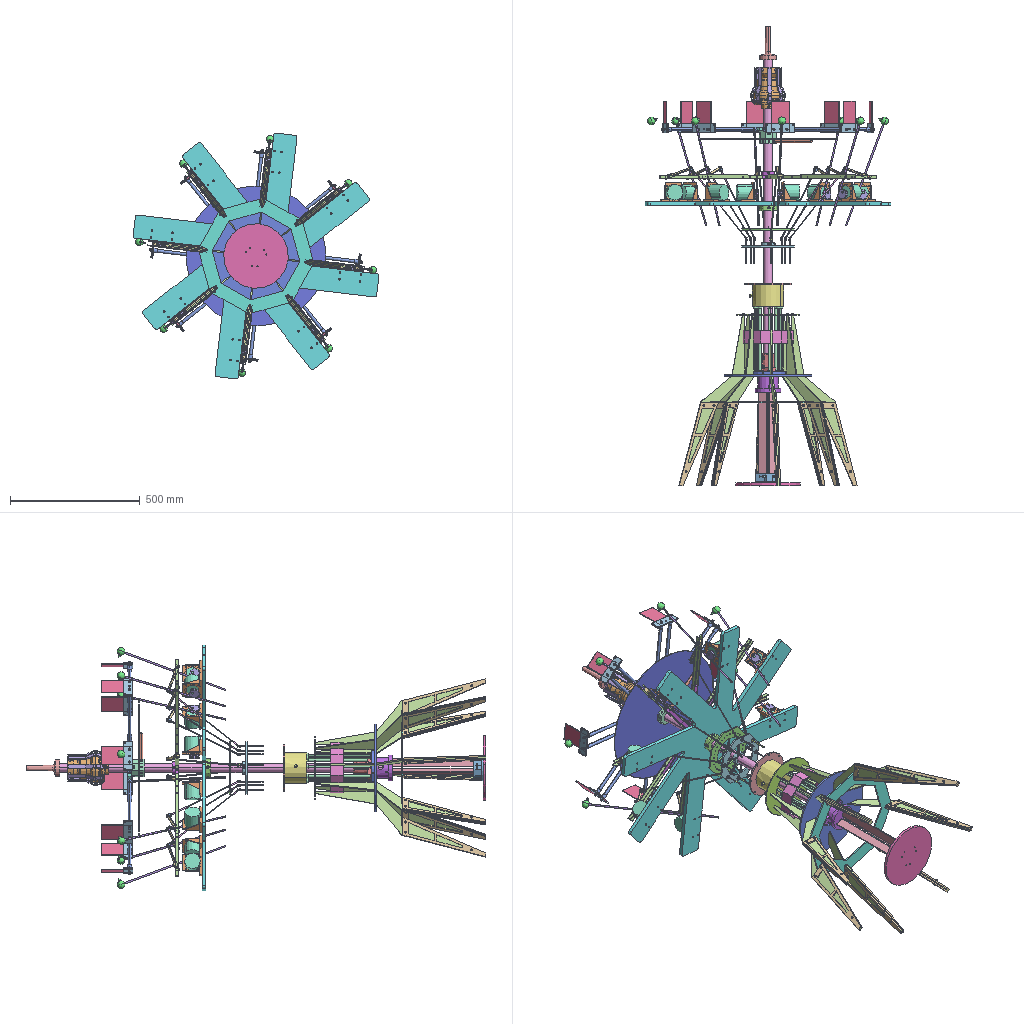Assembly | SolidWorks | 59 different items | 220 placed | box 948 x 1774 x 948 mm
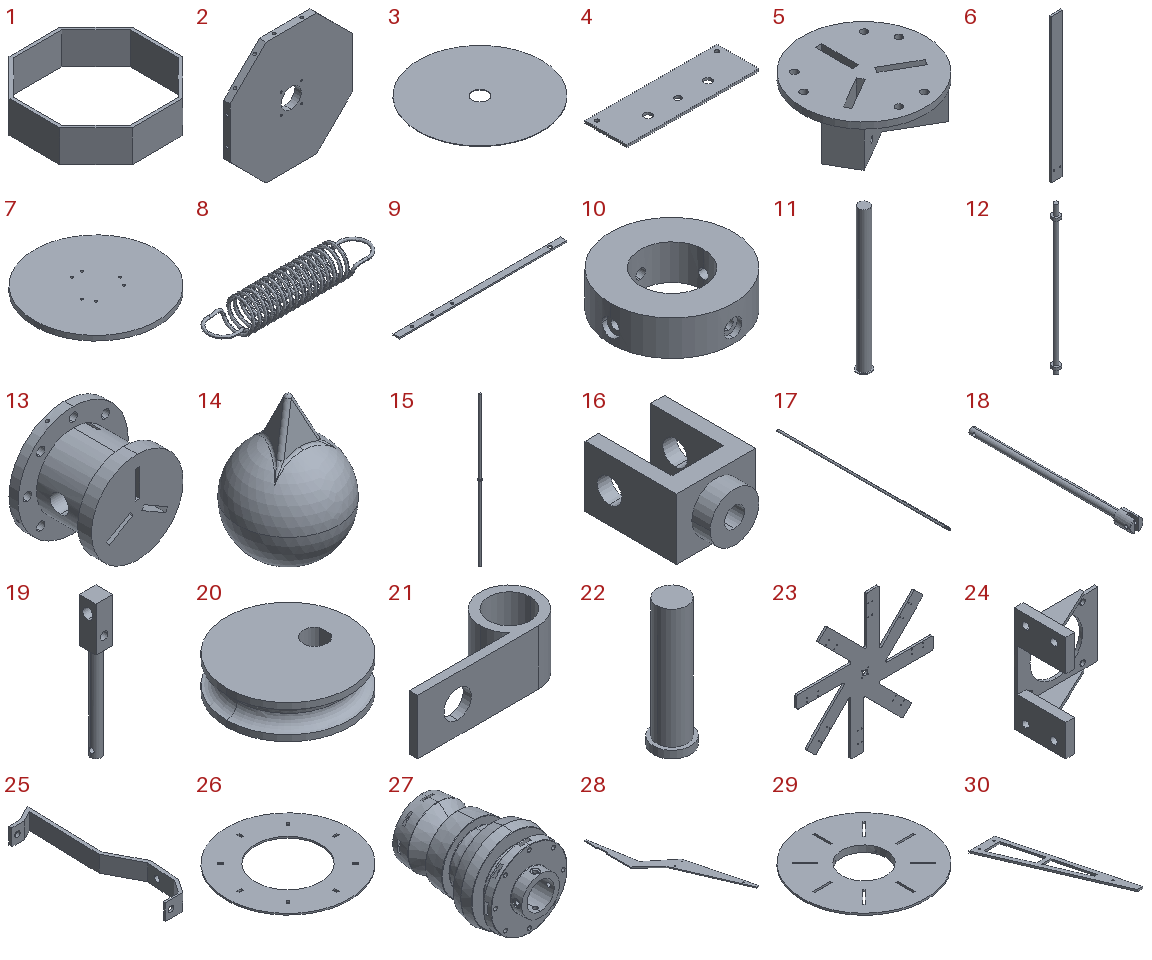Parts list (item | name | quantity | size | volume | features):
1 | - | x1 | 192.167 x 192.167 x 50 mm | 155054 mm3 | features Extrusion 1, ICE 1
2 | - | x1 | 220 x 12 x 220 mm | 463430 mm3 | features ICE 3, CirPattern 2, 3DProfileFeature 1, HoleWzd 1, Revolution 1
3 | - | x1 | 540 x 540 x 2 mm | 450713 mm3 | features Extrusion 1
4 | - | x16 | 110 x 35 x 2 mm | 7490 mm3 | features ICE 3, Extrusion 1
5 | - | x1 | 100 x 100 x 35 mm | 118431 mm3 | features ICE 6, CirPattern 2, Extrusion 1
6 | - | x3 | 30 x 5 x 375 mm | 56098 mm3 | features ICE 4, Cut 1, Extrusion 1, MirrorSolid 1
7 | - | x1 | 250 x 250 x 10 mm | 490035 mm3 | features 3DProfileFeature 1, CirPattern 1, Extrusion 1, HoleWzd 1
8 | - | x1 | 56.999 x 11.387 x 10.999 mm | 441.954 mm3 | features 3DProfileFeature 2, CirPattern 1, CombineBodies 1, Helix 1, ICE 1, Sweep 1
9 | - | x16 | 375 x 14 x 3 mm | 15385 mm3 | features Extrusion 1, ICE 1
10 | - | x1 | 70 x 70 x 20 mm | 54005 mm3 | features CirPattern 2, ICE 2, 3DProfileFeature 1, Extrusion 1, HoleWzd 1
11 | - | x1 | 12.5 x 12.5 x 131 mm | 10333 mm3 | features Extrusion 1, ICE 1
12 | - | x8 | 15 x 15 x 280 mm | 15339 mm3 | features ICE 2, Extrusion 1
13 | - | x1 | 120 x 80 x 120 mm | 422687 mm3 | features ICE 6, CirPattern 3, 3DProfileFeature 2, HoleWzd 2, Revolution 1
14 | - | x8 | 30 x 29.697 x 41.877 mm | 14099 mm3 | features Fillet 2, Blend 1, ICE 1, Revolution 1
15 | - | x8 | 10 x 10 x 430 mm | 12309 mm3 | features ICE 1, Revolution 1
16 | - | x8 | 13 x 18 x 10 mm | 972.93 mm3 | features ICE 3, 3DProfileFeature 1, Extrusion 1, HoleWzd 1
17 | - | x8 | 4 x 340 x 4 mm | 4216 mm3 | features ICE 2, Extrusion 1, Fillet 1
18 | - | x8 | 8 x 100 x 8 mm | 1520 mm3 | features ICE 4, Fillet 2, Extrusion 1
19 | - | x8 | 13 x 13 x 110 mm | 8567 mm3 | features ICE 5, Extrusion 1
20 | - | x8 | 36.4 x 36.4 x 15 mm | 8786 mm3 | features 3DProfileFeature 1, Extrusion 1, HoleWzd 1, ICE 1, Revolution 1
21 | - | x1 | 18 x 7 x 6.6 mm | 200.425 mm3 | features Extrusion 1, ICE 1
22 | - | x1 | 5 x 5 x 17 mm | 220.697 mm3 | features Extrusion 1, ICE 1
23 | - | x1 | 960 x 14 x 960 mm | 4425527 mm3 | features ICE 7, CirPattern 3, Fillet 3, Extrusion 1
24 | - | x8 | 76.5 x 49 x 100 mm | 36422 mm3 | features ICE 5, Extrusion 1, MirrorPattern 1
25 | - | x8 | 37.394 x 139.343 x 15 mm | 7600 mm3 | features ICE 4, Extrusion 1, RevCut 1
26 | - | x1 | 245 x 245 x 3 mm | 100531 mm3 | features CirPattern 1, Extrusion 1, ICE 1
27 | - | x1 | 111.982 x 158 x 111.982 mm | 684523 mm3 | features ICE 7, CirPattern 2, Fillet 1, Revolution 1
28 | - | x8 | 255 x 663 x 5 mm | 131784 mm3 | features Cut 1, Extrusion 1, ICE 1
29 | - | x1 | 340 x 340 x 18 mm | 438812 mm3 | features CirPattern 2, ICE 2, Extrusion 1, RevCut 1
30 | - | x16 | 152.846 x 320 x 5 mm | 40320 mm3 | features ICE 3, Extrusion 1
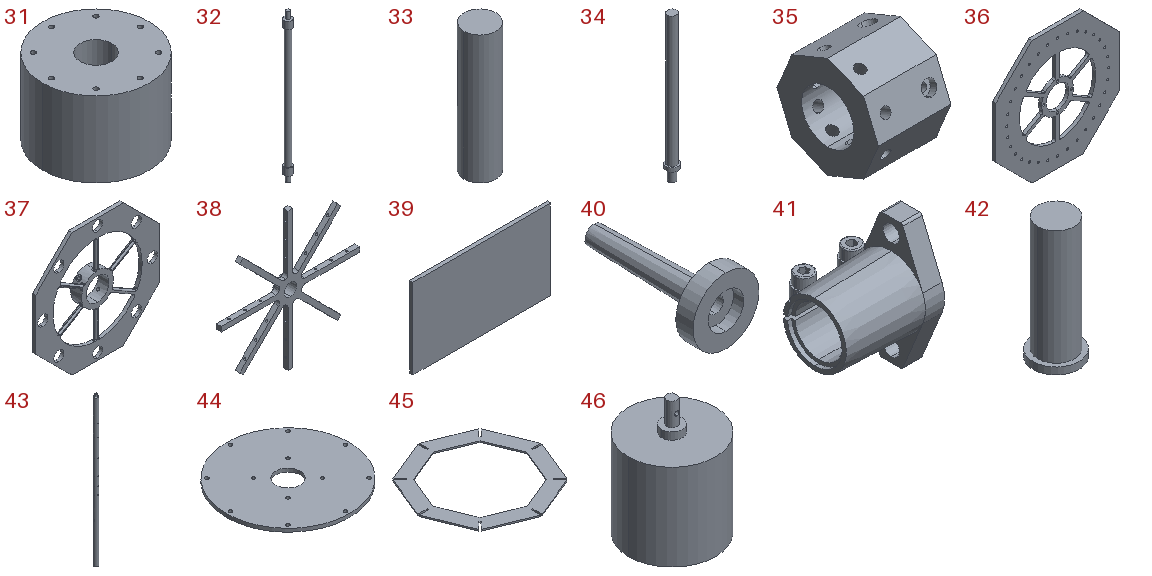31 | - | x1 | 120 x 120 x 85 mm | 867746 mm3 | features 3DProfileFeature 2, CirPattern 2, HoleWzd 2, Extrusion 1, ICE 1
32 | - | x16 | 16 x 16 x 315 mm | 36203 mm3 | features ICE 4, Extrusion 1
33 | - | x9 | 5 x 5 x 20 mm | 392.699 mm3 | features Extrusion 1
34 | - | x1 | 16 x 16 x 195 mm | 21752 mm3 | features ICE 2, Extrusion 1
35 | - | x1 | 50 x 70 x 70 mm | 115293 mm3 | features CirPattern 3, 3DProfileFeature 2, HoleWzd 2, ICE 2, Extrusion 1
36 | - | x1 | 194.015 x 5 x 194.015 mm | 108020 mm3 | features ICE 7, CirPattern 4, Extrusion 1, Fillet 1
37 | - | x1 | - | 92425 mm3 | features ICE 5, CirPattern 3, Fillet 2, Extrusion 1
38 | - | x1 | 400 x 26 x 400 mm | 303636 mm3 | features ICE 6, CirPattern 2, Extrusion 1, Fillet 1
39 | - | x8 | 120 x 3 x 70 mm | 25200 mm3 | features Extrusion 1
40 | - | x1 | 65 x 130 x 65 mm | 88701 mm3 | features ICE 2, Revolution 1
41 | - | x1 | 70 x 58 x 92 mm | 80173 mm3 | features BaseBody 3
42 | - | x1 | 10 x 10 x 26.5 mm | 1374 mm3 | features Extrusion 1, ICE 1
43 | - | x1 | 35 x 35 x 1273 mm | 1203146 mm3 | features ICE 5, LPattern 4, 3DProfileFeature 2, CirPattern 2, HoleWzd 2, Chamfer 1, Extrusion 1
44 | - | x1 | 182 x 182 x 5 mm | 123899 mm3 | features CirPattern 2, ICE 2, Extrusion 1
45 | - | x1 | 447.763 x 447.763 x 5 mm | 295555 mm3 | features ICE 2, Extrusion 1
46 | - | x8 | 60 x 60 x 81 mm | 170965 mm3 | features ICE 4, Extrusion 1
47 | angular contact ball bearings gb | x1 | - | - | -
48 | circlips for hole--type b gb | x1 | - | - | -
49 | cross recessed hex bolts indentation gb | x1 | - | - | -
50 | hex bolts with split pin hole-grade ab gb | x1 | - | - | -
51 | hex head bolts-full thread grade c gb | x1 | - | - | -
52 | hex nut-fine pitch-style washer-grade ab gb | x1 | - | - | -
53 | hex nuts 1-fine pitch-grades ab gb | x1 | - | - | -
54 | hex nuts, style 1-grades ab gb | x1 | - | - | -
55 | hex nuts, style 2-grades ab gb | x1 | - | - | -
56 | hex nuts-style normal-grades ab gb | x1 | - | - | -
57 | hex socket set screws with flat point gb | x1 | - | - | -
58 | hexagon head wood screws gb | x1 | - | - | -
59 | hexagon socket head cap screws gb | x1 | - | - | -
Mates (type | each side: item.copy, entity, surface, feature):
Concentric | 43.1 face cylinder Boss-Extrude 1 | 27.1 face cylinder Revolve 1
Concentric | 40.1 face cylinder Cut-Extrude 1 | 43.1 face cylinder Boss-Extrude 2
Symmetric | 27.1 face plane Cut-Extrude 1 | 27.1 face plane Cut-Extrude 1 | 25.1 plane
Coincident | 27.1 face plane Cut-Extrude 1 | 25.1 face plane Boss-Extrude 2
Coincident | 27.1 face cylinder Cut-Extrude 2 | 25.1 edge
Concentric | 27.1 face cylinder Cut-Extrude 2 | 33.1 face cylinder Boss-Extrude 1
DistanceDim | 33.1 face plane Boss-Extrude 1 | 27.1 face plane Revolve 1
Concentric | 27.1 face cylinder Cut-Extrude 3 | 33.2 face cylinder Boss-Extrude 1
Coincident | 27.1 face plane Revolve 1 | 33.2 face plane Boss-Extrude 1
Concentric | 32.1 face cylinder Boss-Extrude 1 | 2.1 face cylinder M6x1.0 Tapped Hole 1
Coincident | 32.1 face plane Boss-Extrude 2 | 2.1 face plane Cut-Extrude 1
Concentric | 2.1 face cylinder M6x1.0 Tapped Hole 1 | 32.2 face cylinder Boss-Extrude 2
Coincident | 32.1 face plane Boss-Extrude 3 | 32.2 face plane Boss-Extrude 3
Coincident | 2.1 plane | 27.1 plane
Concentric | 32.1 face cylinder Boss-Extrude 5 | 4.1 face cylinder Boss-Extrude 1
Coincident | 32.1 face plane Boss-Extrude 4 | 4.1 face plane Boss-Extrude 1
Concentric | 32.2 face cylinder Boss-Extrude 5 | 4.1 face cylinder Boss-Extrude 1
Coincident | 39.1 face plane Boss-Extrude 1 | 4.1 face plane Boss-Extrude 1 | 2 times
Symmetric | 39.1 face plane Boss-Extrude 1 | 39.1 face plane Boss-Extrude 1 | 4.1 plane
Concentric | 32.2 face cylinder Boss-Extrude 5 | 4.2 face cylinder Boss-Extrude 1
Coincident | 39.1 face plane Boss-Extrude 1 | 4.2 face plane Boss-Extrude 1
Concentric | 32.1 face cylinder Boss-Extrude 5 | 4.2 face cylinder Boss-Extrude 1
Concentric | 43.1 face cylinder Boss-Extrude 1 | 38.1 face cylinder Boss-Extrude 4
Coincident | 43.1 plane | 2.1 plane
Concentric | 43.1 face cylinder Boss-Extrude 1 | 35.1 face cylinder Boss-Extrude 1
Concentric | 35.1 face cylinder CirPattern 1 | 34.1 face cylinder Boss-Extrude 1
Coincident | 35.1 face plane Boss-Extrude 1 | 34.1 face plane Boss-Extrude 2
Concentric | 43.1 face cylinder Boss-Extrude 1 | 3.1 face cylinder Boss-Extrude 1
Tangent | 34.1 face cylinder Boss-Extrude 3 | 3.1 face plane Boss-Extrude 1
Parallel | 2.1 face plane Cut-Extrude 1 | 38.1 face plane Boss-Extrude 5
Concentric | 38.1 face cylinder Cut-Extrude 1 | 9.1 face cylinder Boss-Extrude 1 | 2 times
Coincident | 38.1 face plane Boss-Extrude 5 | 9.1 face plane Boss-Extrude 1
Coincident | 38.1 face plane Boss-Extrude 5 | 9.2 face plane Boss-Extrude 1
Concentric | 38.1 face cylinder Cut-Extrude 1 | 9.2 face cylinder Boss-Extrude 1 | 2 times
DistanceDim | 38.1 face plane Boss-Extrude 4 | 23.1 face plane Boss-Extrude 4
Concentric | 9.2 face cylinder Cut-Extrude 1 | 19.1 face cylinder Cut-Extrude 2
Concentric | 19.1 face cylinder Cut-Extrude 1 | 15.1 face cylinder Revolve 1
Parallel | 9.1 face plane Boss-Extrude 1 | 15.1 plane
Symmetric | 9.1 face plane Boss-Extrude 1 | 9.2 face plane Boss-Extrude 1 | 19.1 plane
Concentric | 43.1 face cylinder Boss-Extrude 1 | 44.1 face cylinder Boss-Extrude 1
Concentric | 18.1 face cylinder Cut-Extrude 7 | 17.1 face cylinder Cut-Extrude 6
Symmetric | 18.1 face plane Cut-Extrude 5 | 18.1 face plane Cut-Extrude 5 | 17.1 plane
Coincident | 16.1 face plane Cut-Extrude 1 | 17.1 face plane Boss-Extrude 3
Concentric | 19.1 face cylinder Cut-Extrude 3 | 16.1 face cylinder Cut-Extrude 2
Symmetric | 19.1 plane | 16.1 face plane Cut-Extrude 1 | 16.1 face plane Cut-Extrude 1
Parallel | 16.1 face plane Boss-Extrude 1 | 17.1 plane
Concentric | 44.1 face cylinder Cut-Extrude 1 | 18.1 face cylinder Boss-Extrude 3
DistanceDim | 40.1 face plane Revolve 1 | 27.1 face plane Revolve 1
Concentric | 46.1 face cylinder Boss-Extrude 1 | 24.1 face cylinder Cut-Extrude 1
Coincident | 46.1 face plane Boss-Extrude 1 | 24.1 face plane Boss-Extrude 2
Coincident | 23.1 face plane Boss-Extrude 4 | 24.1 face plane Boss-Extrude 1
Concentric | 46.1 face cylinder Boss-Extrude 3 | 20.1 face cylinder Boss-Extrude 1
Coincident | 19.1 face plane Boss-Extrude 1 | 15.1 face plane Boss-Extrude 1
Coincident | 46.1 face plane Boss-Extrude 3 | 20.1 face plane Boss-Extrude 1
Concentric | 43.1 face cylinder Boss-Extrude 1 | 23.1 face cylinder Boss-Extrude 4
Parallel | 43.1 plane | 23.1 face plane Boss-Extrude 5
Tangent | 15.1 face cylinder Revolve 1 | 20.1 face torus Revolve 1
Concentric | 23.1 face cylinder Cut-Extrude 7 | 24.1 face cylinder Boss-Extrude 1 | 2 times
Concentric | 43.1 face cylinder Boss-Extrude 1 | 36.1 face cylinder Boss-Extrude 1
Concentric | 36.1 face cylinder Cut-Extrude 3 | 21.1 face cylinder Cut-Extrude 1
Coincident | 36.1 face plane Boss-Extrude 1 | 21.1 face plane Boss-Extrude 1
Parallel | 38.1 face plane CirPattern 1 | 36.1 face plane Boss-Extrude 1
Concentric | 43.1 face cylinder Boss-Extrude 1 | 37.1 face cylinder Boss-Extrude 1
Parallel | 36.1 face plane Boss-Extrude 1 | 37.1 face plane Boss-Extrude 1
DistanceDim | 36.1 face plane Boss-Extrude 1 | 37.1 face plane Boss-Extrude 1
DistanceDim | 37.1 face plane Boss-Extrude 1 | 44.1 face plane Boss-Extrude 1
Concentric | 43.1 face cylinder Boss-Extrude 1 | 31.1 face cylinder Boss-Extrude 1
Coincident | 44.1 face plane Boss-Extrude 1 | 31.1 face plane Boss-Extrude 1
Concentric | 26.1 face cylinder Boss-Extrude 1 | 43.1 face cylinder Boss-Extrude 1
Concentric | 43.1 face cylinder Boss-Extrude 1 | 13.1 face cylinder Revolve 1
Concentric | 31.1 face cylinder M6x1.0 Tapped Hole 1 | 12.1 face cylinder Boss-Extrude 1
DistanceDim | 12.1 face plane Boss-Extrude 1 | 31.1 face plane Boss-Extrude 1
Coincident | 13.1 face plane Revolve 1 | 12.1 face plane Boss-Extrude 2
Concentric | 13.1 face cylinder CirPattern 1 | 12.1 face cylinder Boss-Extrude 1
Concentric | 43.1 face cylinder Boss-Extrude 1 | 29.1 face cylinder Boss-Extrude 1
Coincident | 26.1 face plane Cut-Extrude 1 | 28.1 face plane Boss-Extrude 1 | 2 times
DistanceDim | 28.1 face plane Boss-Extrude 1 | 26.1 face plane Boss-Extrude 1
Concentric | 43.1 face cylinder Boss-Extrude 1 | 1.1 select_type:24
Coincident | 28.1 face plane Boss-Extrude 1 | 1.1 face plane Boss-Extrude 1
Symmetric | 28.1 face plane Boss-Extrude 1 | 28.1 face plane Boss-Extrude 1 | 1.1 plane
Symmetric | 43.1 plane | 28.1 face plane Boss-Extrude 1 | 28.1 face plane Boss-Extrude 1
Symmetric | 13.1 plane | 28.1 face plane Boss-Extrude 1 | 28.1 face plane Boss-Extrude 1
Coincident | 29.1 face plane Cut-Extrude 1 | 28.1 face plane Boss-Extrude 1
Coincident | 29.1 face plane Boss-Extrude 1 | 28.1 edge
Concentric | 43.1 face cylinder Boss-Extrude 1 | 45.1 select_type:24
Symmetric | 28.1 face plane Boss-Extrude 1 | 28.1 face plane Boss-Extrude 1 | 45.1 plane
Coincident | 28.1 face plane Boss-Extrude 1 | 30.1 face plane Boss-Extrude 1 | 3 times
Coincident | 45.1 face plane Boss-Extrude 1 | 30.1 face plane Boss-Extrude 1
Coincident | 28.1 face plane Boss-Extrude 1 | 30.2 face plane Boss-Extrude 1 | 2 times
Concentric | 28.1 face cylinder Cut-Extrude 1 | 30.2 face cylinder Cut-Extrude 1
Coincident | 13.1 face plane Cut-Extrude 2 | 6.1 face plane Boss-Extrude 1 | 2 times
Concentric | 13.1 face cylinder Revolve 1 | 5.1 face cylinder Boss-Extrude 1
Concentric | 31.1 face cylinder Cut-Extrude 1 | 11.1 face cylinder Boss-Extrude 1
Tangent | 31.1 face cylinder Boss-Extrude 1 | 11.1 face plane Boss-Extrude 2
Coincident | 16.1 edge | 22.1 face cylinder Boss-Extrude 2
Coincident | 16.1 face plane Boss-Extrude 1 | 22.1 face plane Boss-Extrude 1
Concentric | 9.1 face cylinder Cut-Extrude 1 | 42.1 face cylinder Boss-Extrude 2
Coincident | 9.2 face plane Boss-Extrude 1 | 42.1 face plane Boss-Extrude 1
Concentric | 43.1 face cylinder LPattern 3 | 35.1 face cylinder Cut-Extrude 2
Coincident | 2.1 face plane Revolve 1 | 35.1 face plane Boss-Extrude 1
Concentric | 2.1 face cylinder CirPattern 2 | 35.1 face cylinder M3x0.5 Tapped Hole 1
Concentric | 2.1 face cylinder CirPattern 2 | 35.1 face cylinder CirPattern 3
Coincident | 40.1 face plane Cut-Extrude 1 | 43.1 face plane Cut-Extrude 2
Concentric | 43.1 face cylinder LPattern 2 | 38.1 face cylinder Cut-Extrude 2
Concentric | 13.1 face cylinder CirPattern 4 | 29.1 face cylinder CirPattern 2
Concentric | 16.1 face cylinder Boss-Extrude 2 | 17.1 face cylinder Boss-Extrude 3
Concentric | 43.1 face cylinder Boss-Extrude 1 | 10.1 face cylinder Boss-Extrude 1
Concentric | 43.1 face cylinder CirPattern 2 | 10.1 face cylinder CirPattern 1
Coincident | 6.1 face plane Mirror 2 | 5.1 face plane Boss-Extrude 1
Coincident | 5.1 face plane Boss-Extrude 1 | 6.2 face plane Mirror 2
Coincident | 5.1 face plane Boss-Extrude 1 | 6.2 face plane Boss-Extrude 1
Coincident | 5.1 face plane Boss-Extrude 1 | 7.1 face plane Boss-Extrude 1
Concentric | 5.1 face cylinder Boss-Extrude 1 | 7.1 face cylinder Boss-Extrude 1
Concentric | 5.1 face cylinder Cut-Extrude 3 | 7.1 face cylinder CirPattern 1
Coincident | 13.1 face plane Cut-Extrude 2 | 6.1 face plane Boss-Extrude 2
Coincident | 13.1 face plane CirPattern 3 | 6.2 face plane Boss-Extrude 2
Concentric | 43.1 face cylinder Boss-Extrude 1 | 41.1 face cone SHFTL35_b-1-solid1
Coincident | 13.1 face plane Revolve 1 | 41.1 face plane SHFTL35_b-1-solid1
Concentric | 13.1 face cylinder M10x1.0 Tapped Hole 1 | 41.1 face cylinder SHFTL35_b-1-solid1
Coincident | 5.1 face plane Boss-Extrude 1 | 6.3 face plane Boss-Extrude 2
Parallel | 5.1 face plane Boss-Extrude 1 | 6.3 face plane Boss-Extrude 1